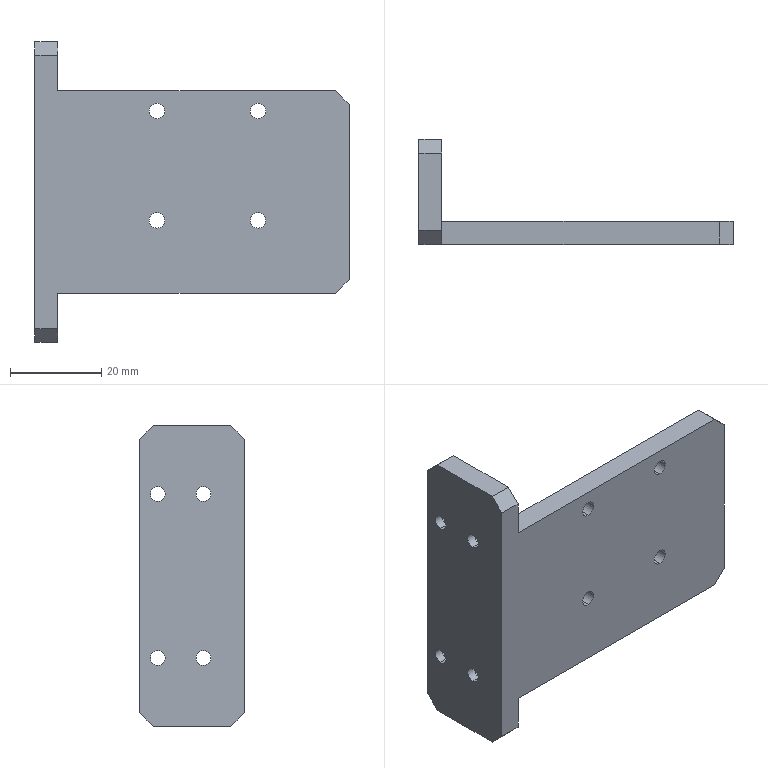Part | STEP file | Guide wheel mechanism revised.sldasm-Part-497 | 1 solid | 44 faces | box 69 x 23 x 66 mm | volume 21162 mm3 | cylinder 24 | plane 20 | commonest cylinder face diameters 3.24 x8 3.4 x8 5.5 x8
STEP:
#1=CARTESIAN_POINT('',(-3.,4.,20.75));
#2=VERTEX_POINT('',#1);
#3=CARTESIAN_POINT('',(-3.,4.,15.25));
#4=VERTEX_POINT('',#3);
#5=CARTESIAN_POINT('',(-3.,4.,18.));
#6=DIRECTION('',(1.,0.,0.));
#7=DIRECTION('',(0.,0.,-1.));
#8=AXIS2_PLACEMENT_3D('',#5,#6,#7);
#9=CIRCLE('',#8,2.75);
#10=EDGE_CURVE('',#2,#4,#9,.T.);
#11=ORIENTED_EDGE('',*,*,#10,.F.);
#12=CARTESIAN_POINT('',(0.,4.,20.75));
#13=VERTEX_POINT('',#12);
#14=CARTESIAN_POINT('',(-3.,4.,20.75));
#15=DIRECTION('',(1.,0.,0.));
#16=VECTOR('',#15,1000.);
#17=LINE('',#14,#16);
#18=EDGE_CURVE('',#2,#13,#17,.T.);
#19=ORIENTED_EDGE('',*,*,#18,.T.);
#20=CARTESIAN_POINT('',(0.,4.,15.25));
#21=VERTEX_POINT('',#20);
#22=CARTESIAN_POINT('',(0.,4.,18.));
#23=DIRECTION('',(1.,0.,0.));
#24=DIRECTION('',(0.,0.,-1.));
#25=AXIS2_PLACEMENT_3D('',#22,#23,#24);
#26=CIRCLE('',#25,2.75);
#27=EDGE_CURVE('',#13,#21,#26,.T.);
#28=ORIENTED_EDGE('',*,*,#27,.T.);
#29=CARTESIAN_POINT('',(-3.,4.,15.25));
#30=DIRECTION('',(1.,0.,0.));
#31=VECTOR('',#30,1000.);
#32=LINE('',#29,#31);
#33=EDGE_CURVE('',#4,#21,#32,.T.);
#34=ORIENTED_EDGE('',*,*,#33,.F.);
#35=EDGE_LOOP('',(#11,#19,#28,#34));
#36=FACE_OUTER_BOUND('',#35,.T.);
#37=CARTESIAN_POINT('',(-3.,4.,18.));
#38=DIRECTION('',(1.,0.,0.));
#39=DIRECTION('',(0.,0.,-1.));
#40=AXIS2_PLACEMENT_3D('',#37,#38,#39);
#41=CYLINDRICAL_SURFACE('',#40,2.75);
#42=ADVANCED_FACE('',(#36),#41,.F.);
#43=CARTESIAN_POINT('',(-3.,4.,-15.25));
#44=VERTEX_POINT('',#43);
#45=CARTESIAN_POINT('',(-3.,4.,-20.75));
#46=VERTEX_POINT('',#45);
#47=CARTESIAN_POINT('',(-3.,4.,-18.));
#48=DIRECTION('',(1.,0.,0.));
#49=DIRECTION('',(0.,0.,-1.));
#50=AXIS2_PLACEMENT_3D('',#47,#48,#49);
#51=CIRCLE('',#50,2.75);
#52=EDGE_CURVE('',#44,#46,#51,.T.);
#53=ORIENTED_EDGE('',*,*,#52,.F.);
#54=CARTESIAN_POINT('',(0.,4.,-15.25));
#55=VERTEX_POINT('',#54);
#56=CARTESIAN_POINT('',(-3.,4.,-15.25));
#57=DIRECTION('',(1.,0.,0.));
#58=VECTOR('',#57,1000.);
#59=LINE('',#56,#58);
#60=EDGE_CURVE('',#44,#55,#59,.T.);
#61=ORIENTED_EDGE('',*,*,#60,.T.);
#62=CARTESIAN_POINT('',(0.,4.,-20.75));
#63=VERTEX_POINT('',#62);
#64=CARTESIAN_POINT('',(0.,4.,-18.));
#65=DIRECTION('',(1.,0.,0.));
#66=DIRECTION('',(0.,0.,-1.));
#67=AXIS2_PLACEMENT_3D('',#64,#65,#66);
#68=CIRCLE('',#67,2.75);
#69=EDGE_CURVE('',#55,#63,#68,.T.);
#70=ORIENTED_EDGE('',*,*,#69,.T.);
#71=CARTESIAN_POINT('',(-3.,4.,-20.75));
#72=DIRECTION('',(1.,0.,0.));
#73=VECTOR('',#72,1000.);
#74=LINE('',#71,#73);
#75=EDGE_CURVE('',#46,#63,#74,.T.);
#76=ORIENTED_EDGE('',*,*,#75,.F.);
#77=EDGE_LOOP('',(#53,#61,#70,#76));
#78=FACE_OUTER_BOUND('',#77,.T.);
#79=CARTESIAN_POINT('',(-3.,4.,-18.));
#80=DIRECTION('',(1.,0.,0.));
#81=DIRECTION('',(0.,0.,-1.));
#82=AXIS2_PLACEMENT_3D('',#79,#80,#81);
#83=CYLINDRICAL_SURFACE('',#82,2.75);
#84=ADVANCED_FACE('',(#78),#83,.F.);
#85=CARTESIAN_POINT('',(-3.,14.,-15.25));
#86=VERTEX_POINT('',#85);
#87=CARTESIAN_POINT('',(-3.,14.,-20.75));
#88=VERTEX_POINT('',#87);
#89=CARTESIAN_POINT('',(-3.,14.,-18.));
#90=DIRECTION('',(1.,0.,0.));
#91=DIRECTION('',(0.,0.,-1.));
#92=AXIS2_PLACEMENT_3D('',#89,#90,#91);
#93=CIRCLE('',#92,2.75);
#94=EDGE_CURVE('',#86,#88,#93,.T.);
#95=ORIENTED_EDGE('',*,*,#94,.F.);
#96=CARTESIAN_POINT('',(0.,14.,-15.25));
#97=VERTEX_POINT('',#96);
#98=CARTESIAN_POINT('',(-3.,14.,-15.25));
#99=DIRECTION('',(1.,0.,0.));
#100=VECTOR('',#99,1000.);
#101=LINE('',#98,#100);
#102=EDGE_CURVE('',#86,#97,#101,.T.);
#103=ORIENTED_EDGE('',*,*,#102,.T.);
#104=CARTESIAN_POINT('',(0.,14.,-20.75));
#105=VERTEX_POINT('',#104);
#106=CARTESIAN_POINT('',(0.,14.,-18.));
#107=DIRECTION('',(1.,0.,0.));
#108=DIRECTION('',(0.,0.,-1.));
#109=AXIS2_PLACEMENT_3D('',#106,#107,#108);
#110=CIRCLE('',#109,2.75);
#111=EDGE_CURVE('',#97,#105,#110,.T.);
#112=ORIENTED_EDGE('',*,*,#111,.T.);
#113=CARTESIAN_POINT('',(-3.,14.,-20.75));
#114=DIRECTION('',(1.,0.,0.));
#115=VECTOR('',#114,1000.);
#116=LINE('',#113,#115);
#117=EDGE_CURVE('',#88,#105,#116,.T.);
#118=ORIENTED_EDGE('',*,*,#117,.F.);
#119=EDGE_LOOP('',(#95,#103,#112,#118));
#120=FACE_OUTER_BOUND('',#119,.T.);
#121=CARTESIAN_POINT('',(-3.,14.,-18.));
#122=DIRECTION('',(1.,0.,0.));
#123=DIRECTION('',(0.,0.,-1.));
#124=AXIS2_PLACEMENT_3D('',#121,#122,#123);
#125=CYLINDRICAL_SURFACE('',#124,2.75);
#126=ADVANCED_FACE('',(#120),#125,.F.);
#127=CARTESIAN_POINT('',(-3.,14.,20.75));
#128=VERTEX_POINT('',#127);
#129=CARTESIAN_POINT('',(-3.,14.,15.25));
#130=VERTEX_POINT('',#129);
#131=CARTESIAN_POINT('',(-3.,14.,18.));
#132=DIRECTION('',(1.,0.,0.));
#133=DIRECTION('',(0.,0.,-1.));
#134=AXIS2_PLACEMENT_3D('',#131,#132,#133);
#135=CIRCLE('',#134,2.75);
#136=EDGE_CURVE('',#128,#130,#135,.T.);
#137=ORIENTED_EDGE('',*,*,#136,.F.);
#138=CARTESIAN_POINT('',(0.,14.,20.75));
#139=VERTEX_POINT('',#138);
#140=CARTESIAN_POINT('',(-3.,14.,20.75));
#141=DIRECTION('',(1.,0.,0.));
#142=VECTOR('',#141,1000.);
#143=LINE('',#140,#142);
#144=EDGE_CURVE('',#128,#139,#143,.T.);
#145=ORIENTED_EDGE('',*,*,#144,.T.);
#146=CARTESIAN_POINT('',(0.,14.,15.25));
#147=VERTEX_POINT('',#146);
#148=CARTESIAN_POINT('',(0.,14.,18.));
#149=DIRECTION('',(1.,0.,0.));
#150=DIRECTION('',(0.,0.,-1.));
#151=AXIS2_PLACEMENT_3D('',#148,#149,#150);
#152=CIRCLE('',#151,2.75);
#153=EDGE_CURVE('',#139,#147,#152,.T.);
#154=ORIENTED_EDGE('',*,*,#153,.T.);
#155=CARTESIAN_POINT('',(-3.,14.,15.25));
#156=DIRECTION('',(1.,0.,0.));
#157=VECTOR('',#156,1000.);
#158=LINE('',#155,#157);
#159=EDGE_CURVE('',#130,#147,#158,.T.);
#160=ORIENTED_EDGE('',*,*,#159,.F.);
#161=EDGE_LOOP('',(#137,#145,#154,#160));
#162=FACE_OUTER_BOUND('',#161,.T.);
#163=CARTESIAN_POINT('',(-3.,14.,18.));
#164=DIRECTION('',(1.,0.,0.));
#165=DIRECTION('',(0.,0.,-1.));
#166=AXIS2_PLACEMENT_3D('',#163,#164,#165);
#167=CYLINDRICAL_SURFACE('',#166,2.75);
#168=ADVANCED_FACE('',(#162),#167,.F.);
#169=CARTESIAN_POINT('',(21.8,-5.,16.05));
#170=VERTEX_POINT('',#169);
#171=CARTESIAN_POINT('',(21.8,-5.,19.45));
#172=VERTEX_POINT('',#171);
#173=CARTESIAN_POINT('',(21.8,-5.,17.75));
#174=DIRECTION('',(0.,1.,0.));
#175=DIRECTION('',(0.,0.,-1.));
#176=AXIS2_PLACEMENT_3D('',#173,#174,#175);
#177=CIRCLE('',#176,1.7);
#178=EDGE_CURVE('',#170,#172,#177,.T.);
#179=ORIENTED_EDGE('',*,*,#178,.F.);
#180=CARTESIAN_POINT('',(21.8,0.,16.05));
#181=VERTEX_POINT('',#180);
#182=CARTESIAN_POINT('',(21.8,-5.001,16.05));
#183=DIRECTION('',(0.,1.,0.));
#184=VECTOR('',#183,1000.);
#185=LINE('',#182,#184);
#186=EDGE_CURVE('',#170,#181,#185,.T.);
#187=ORIENTED_EDGE('',*,*,#186,.T.);
#188=CARTESIAN_POINT('',(21.8,0.,19.45));
#189=VERTEX_POINT('',#188);
#190=CARTESIAN_POINT('',(21.8,0.,17.75));
#191=DIRECTION('',(0.,1.,0.));
#192=DIRECTION('',(0.,0.,1.));
#193=AXIS2_PLACEMENT_3D('',#190,#191,#192);
#194=CIRCLE('',#193,1.7);
#195=EDGE_CURVE('',#181,#189,#194,.T.);
#196=ORIENTED_EDGE('',*,*,#195,.T.);
#197=CARTESIAN_POINT('',(21.8,-5.001,19.45));
#198=DIRECTION('',(0.,1.,0.));
#199=VECTOR('',#198,1000.);
#200=LINE('',#197,#199);
#201=EDGE_CURVE('',#172,#189,#200,.T.);
#202=ORIENTED_EDGE('',*,*,#201,.F.);
#203=EDGE_LOOP('',(#179,#187,#196,#202));
#204=FACE_OUTER_BOUND('',#203,.T.);
#205=CARTESIAN_POINT('',(21.8,-5.001,17.75));
#206=DIRECTION('',(0.,1.,0.));
#207=DIRECTION('',(0.,0.,1.));
#208=AXIS2_PLACEMENT_3D('',#205,#206,#207);
#209=CYLINDRICAL_SURFACE('',#208,1.7);
#210=ADVANCED_FACE('',(#204),#209,.F.);
#211=CARTESIAN_POINT('',(44.,-5.,16.05));
#212=VERTEX_POINT('',#211);
#213=CARTESIAN_POINT('',(44.,-5.,19.45));
#214=VERTEX_POINT('',#213);
#215=CARTESIAN_POINT('',(44.,-5.,17.75));
#216=DIRECTION('',(0.,1.,0.));
#217=DIRECTION('',(0.,0.,-1.));
#218=AXIS2_PLACEMENT_3D('',#215,#216,#217);
#219=CIRCLE('',#218,1.7);
#220=EDGE_CURVE('',#212,#214,#219,.T.);
#221=ORIENTED_EDGE('',*,*,#220,.F.);
#222=CARTESIAN_POINT('',(44.,0.,16.05));
#223=VERTEX_POINT('',#222);
#224=CARTESIAN_POINT('',(44.,-5.001,16.05));
#225=DIRECTION('',(0.,1.,0.));
#226=VECTOR('',#225,1000.);
#227=LINE('',#224,#226);
#228=EDGE_CURVE('',#212,#223,#227,.T.);
#229=ORIENTED_EDGE('',*,*,#228,.T.);
#230=CARTESIAN_POINT('',(44.,0.,19.45));
#231=VERTEX_POINT('',#230);
#232=CARTESIAN_POINT('',(44.,0.,17.75));
#233=DIRECTION('',(0.,1.,0.));
#234=DIRECTION('',(0.,0.,1.));
#235=AXIS2_PLACEMENT_3D('',#232,#233,#234);
#236=CIRCLE('',#235,1.7);
#237=EDGE_CURVE('',#223,#231,#236,.T.);
#238=ORIENTED_EDGE('',*,*,#237,.T.);
#239=CARTESIAN_POINT('',(44.,-5.001,19.45));
#240=DIRECTION('',(0.,1.,0.));
#241=VECTOR('',#240,1000.);
#242=LINE('',#239,#241);
#243=EDGE_CURVE('',#214,#231,#242,.T.);
#244=ORIENTED_EDGE('',*,*,#243,.F.);
#245=EDGE_LOOP('',(#221,#229,#238,#244));
#246=FACE_OUTER_BOUND('',#245,.T.);
#247=CARTESIAN_POINT('',(44.,-5.001,17.75));
#248=DIRECTION('',(0.,1.,0.));
#249=DIRECTION('',(0.,0.,1.));
#250=AXIS2_PLACEMENT_3D('',#247,#248,#249);
#251=CYLINDRICAL_SURFACE('',#250,1.7);
#252=ADVANCED_FACE('',(#246),#251,.F.);
#253=CARTESIAN_POINT('',(44.,-5.,-7.95));
#254=VERTEX_POINT('',#253);
#255=CARTESIAN_POINT('',(44.,-5.,-4.55));
#256=VERTEX_POINT('',#255);
#257=CARTESIAN_POINT('',(44.,-5.,-6.25));
#258=DIRECTION('',(0.,1.,0.));
#259=DIRECTION('',(0.,0.,-1.));
#260=AXIS2_PLACEMENT_3D('',#257,#258,#259);
#261=CIRCLE('',#260,1.7);
#262=EDGE_CURVE('',#254,#256,#261,.T.);
#263=ORIENTED_EDGE('',*,*,#262,.F.);
#264=CARTESIAN_POINT('',(44.,0.,-7.95));
#265=VERTEX_POINT('',#264);
#266=CARTESIAN_POINT('',(44.,-5.001,-7.95));
#267=DIRECTION('',(0.,1.,0.));
#268=VECTOR('',#267,1000.);
#269=LINE('',#266,#268);
#270=EDGE_CURVE('',#254,#265,#269,.T.);
#271=ORIENTED_EDGE('',*,*,#270,.T.);
#272=CARTESIAN_POINT('',(44.,0.,-4.55));
#273=VERTEX_POINT('',#272);
#274=CARTESIAN_POINT('',(44.,0.,-6.25));
#275=DIRECTION('',(0.,1.,0.));
#276=DIRECTION('',(0.,0.,1.));
#277=AXIS2_PLACEMENT_3D('',#274,#275,#276);
#278=CIRCLE('',#277,1.7);
#279=EDGE_CURVE('',#265,#273,#278,.T.);
#280=ORIENTED_EDGE('',*,*,#279,.T.);
#281=CARTESIAN_POINT('',(44.,-5.001,-4.55));
#282=DIRECTION('',(0.,1.,0.));
#283=VECTOR('',#282,1000.);
#284=LINE('',#281,#283);
#285=EDGE_CURVE('',#256,#273,#284,.T.);
#286=ORIENTED_EDGE('',*,*,#285,.F.);
#287=EDGE_LOOP('',(#263,#271,#280,#286));
#288=FACE_OUTER_BOUND('',#287,.T.);
#289=CARTESIAN_POINT('',(44.,-5.001,-6.25));
#290=DIRECTION('',(0.,1.,0.));
#291=DIRECTION('',(0.,0.,1.));
#292=AXIS2_PLACEMENT_3D('',#289,#290,#291);
#293=CYLINDRICAL_SURFACE('',#292,1.7);
#294=ADVANCED_FACE('',(#288),#293,.F.);
#295=CARTESIAN_POINT('',(21.8,-5.,-7.95));
#296=VERTEX_POINT('',#295);
#297=CARTESIAN_POINT('',(21.8,-5.,-4.55));
#298=VERTEX_POINT('',#297);
#299=CARTESIAN_POINT('',(21.8,-5.,-6.25));
#300=DIRECTION('',(0.,1.,0.));
#301=DIRECTION('',(0.,0.,-1.));
#302=AXIS2_PLACEMENT_3D('',#299,#300,#301);
#303=CIRCLE('',#302,1.7);
#304=EDGE_CURVE('',#296,#298,#303,.T.);
#305=ORIENTED_EDGE('',*,*,#304,.F.);
#306=CARTESIAN_POINT('',(21.8,0.,-7.95));
#307=VERTEX_POINT('',#306);
#308=CARTESIAN_POINT('',(21.8,-5.001,-7.95));
#309=DIRECTION('',(0.,1.,0.));
#310=VECTOR('',#309,1000.);
#311=LINE('',#308,#310);
#312=EDGE_CURVE('',#296,#307,#311,.T.);
#313=ORIENTED_EDGE('',*,*,#312,.T.);
#314=CARTESIAN_POINT('',(21.8,0.,-4.55));
#315=VERTEX_POINT('',#314);
#316=CARTESIAN_POINT('',(21.8,0.,-6.25));
#317=DIRECTION('',(0.,1.,0.));
#318=DIRECTION('',(0.,0.,1.));
#319=AXIS2_PLACEMENT_3D('',#316,#317,#318);
#320=CIRCLE('',#319,1.7);
#321=EDGE_CURVE('',#307,#315,#320,.T.);
#322=ORIENTED_EDGE('',*,*,#321,.T.);
#323=CARTESIAN_POINT('',(21.8,-5.001,-4.55));
#324=DIRECTION('',(0.,1.,0.));
#325=VECTOR('',#324,1000.);
#326=LINE('',#323,#325);
#327=EDGE_CURVE('',#298,#315,#326,.T.);
#328=ORIENTED_EDGE('',*,*,#327,.F.);
#329=EDGE_LOOP('',(#305,#313,#322,#328));
#330=FACE_OUTER_BOUND('',#329,.T.);
#331=CARTESIAN_POINT('',(21.8,-5.001,-6.25));
#332=DIRECTION('',(0.,1.,0.));
#333=DIRECTION('',(0.,0.,1.));
#334=AXIS2_PLACEMENT_3D('',#331,#332,#333);
#335=CYLINDRICAL_SURFACE('',#334,1.7);
#336=ADVANCED_FACE('',(#330),#335,.F.);
#337=CARTESIAN_POINT('',(-5.,14.,19.62));
#338=VERTEX_POINT('',#337);
#339=CARTESIAN_POINT('',(-5.,14.,16.38));
#340=VERTEX_POINT('',#339);
#341=CARTESIAN_POINT('',(-5.,14.,18.));
#342=DIRECTION('',(1.,0.,0.));
#343=DIRECTION('',(0.,0.,1.));
#344=AXIS2_PLACEMENT_3D('',#341,#342,#343);
#345=CIRCLE('',#344,1.62);
#346=EDGE_CURVE('',#338,#340,#345,.T.);
#347=ORIENTED_EDGE('',*,*,#346,.F.);
#348=CARTESIAN_POINT('',(-3.,14.,19.62));
#349=VERTEX_POINT('',#348);
#350=CARTESIAN_POINT('',(-5.001,14.,19.62));
#351=DIRECTION('',(1.,0.,0.));
#352=VECTOR('',#351,1000.);
#353=LINE('',#350,#352);
#354=EDGE_CURVE('',#338,#349,#353,.T.);
#355=ORIENTED_EDGE('',*,*,#354,.T.);
#356=CARTESIAN_POINT('',(-3.,14.,16.38));
#357=VERTEX_POINT('',#356);
#358=CARTESIAN_POINT('',(-3.,14.,18.));
#359=DIRECTION('',(-1.,0.,0.));
#360=DIRECTION('',(0.,0.,-1.));
#361=AXIS2_PLACEMENT_3D('',#358,#359,#360);
#362=CIRCLE('',#361,1.62);
#363=EDGE_CURVE('',#357,#349,#362,.T.);
#364=ORIENTED_EDGE('',*,*,#363,.F.);
#365=CARTESIAN_POINT('',(-5.001,14.,16.38));
#366=DIRECTION('',(1.,0.,0.));
#367=VECTOR('',#366,1000.);
#368=LINE('',#365,#367);
#369=EDGE_CURVE('',#340,#357,#368,.T.);
#370=ORIENTED_EDGE('',*,*,#369,.F.);
#371=EDGE_LOOP('',(#347,#355,#364,#370));
#372=FACE_OUTER_BOUND('',#371,.T.);
#373=CARTESIAN_POINT('',(-5.001,14.,18.));
#374=DIRECTION('',(1.,0.,0.));
#375=DIRECTION('',(0.,0.,-1.));
#376=AXIS2_PLACEMENT_3D('',#373,#374,#375);
#377=CYLINDRICAL_SURFACE('',#376,1.62);
#378=ADVANCED_FACE('',(#372),#377,.F.);
#379=CARTESIAN_POINT('',(-5.,14.,-16.38));
#380=VERTEX_POINT('',#379);
#381=CARTESIAN_POINT('',(-5.,14.,-19.62));
#382=VERTEX_POINT('',#381);
#383=CARTESIAN_POINT('',(-5.,14.,-18.));
#384=DIRECTION('',(1.,0.,0.));
#385=DIRECTION('',(0.,0.,1.));
#386=AXIS2_PLACEMENT_3D('',#383,#384,#385);
#387=CIRCLE('',#386,1.62);
#388=EDGE_CURVE('',#380,#382,#387,.T.);
#389=ORIENTED_EDGE('',*,*,#388,.F.);
#390=CARTESIAN_POINT('',(-3.,14.,-16.38));
#391=VERTEX_POINT('',#390);
#392=CARTESIAN_POINT('',(-5.001,14.,-16.38));
#393=DIRECTION('',(1.,0.,0.));
#394=VECTOR('',#393,1000.);
#395=LINE('',#392,#394);
#396=EDGE_CURVE('',#380,#391,#395,.T.);
#397=ORIENTED_EDGE('',*,*,#396,.T.);
#398=CARTESIAN_POINT('',(-3.,14.,-19.62));
#399=VERTEX_POINT('',#398);
#400=CARTESIAN_POINT('',(-3.,14.,-18.));
#401=DIRECTION('',(-1.,0.,0.));
#402=DIRECTION('',(0.,0.,-1.));
#403=AXIS2_PLACEMENT_3D('',#400,#401,#402);
#404=CIRCLE('',#403,1.62);
#405=EDGE_CURVE('',#399,#391,#404,.T.);
#406=ORIENTED_EDGE('',*,*,#405,.F.);
#407=CARTESIAN_POINT('',(-5.001,14.,-19.62));
#408=DIRECTION('',(1.,0.,0.));
#409=VECTOR('',#408,1000.);
#410=LINE('',#407,#409);
#411=EDGE_CURVE('',#382,#399,#410,.T.);
#412=ORIENTED_EDGE('',*,*,#411,.F.);
#413=EDGE_LOOP('',(#389,#397,#406,#412));
#414=FACE_OUTER_BOUND('',#413,.T.);
#415=CARTESIAN_POINT('',(-5.001,14.,-18.));
#416=DIRECTION('',(1.,0.,0.));
#417=DIRECTION('',(0.,0.,-1.));
#418=AXIS2_PLACEMENT_3D('',#415,#416,#417);
#419=CYLINDRICAL_SURFACE('',#418,1.62);
#420=ADVANCED_FACE('',(#414),#419,.F.);
#421=CARTESIAN_POINT('',(-5.,4.,-16.38));
#422=VERTEX_POINT('',#421);
#423=CARTESIAN_POINT('',(-5.,4.,-19.62));
#424=VERTEX_POINT('',#423);
#425=CARTESIAN_POINT('',(-5.,4.,-18.));
#426=DIRECTION('',(1.,0.,0.));
#427=DIRECTION('',(0.,0.,1.));
#428=AXIS2_PLACEMENT_3D('',#425,#426,#427);
#429=CIRCLE('',#428,1.62);
#430=EDGE_CURVE('',#422,#424,#429,.T.);
#431=ORIENTED_EDGE('',*,*,#430,.F.);
#432=CARTESIAN_POINT('',(-3.,4.,-16.38));
#433=VERTEX_POINT('',#432);
#434=CARTESIAN_POINT('',(-5.001,4.,-16.38));
#435=DIRECTION('',(1.,0.,0.));
#436=VECTOR('',#435,1000.);
#437=LINE('',#434,#436);
#438=EDGE_CURVE('',#422,#433,#437,.T.);
#439=ORIENTED_EDGE('',*,*,#438,.T.);
#440=CARTESIAN_POINT('',(-3.,4.,-19.62));
#441=VERTEX_POINT('',#440);
#442=CARTESIAN_POINT('',(-3.,4.,-18.));
#443=DIRECTION('',(-1.,0.,0.));
#444=DIRECTION('',(0.,0.,-1.));
#445=AXIS2_PLACEMENT_3D('',#442,#443,#444);
#446=CIRCLE('',#445,1.62);
#447=EDGE_CURVE('',#441,#433,#446,.T.);
#448=ORIENTED_EDGE('',*,*,#447,.F.);
#449=CARTESIAN_POINT('',(-5.001,4.,-19.62));
#450=DIRECTION('',(1.,0.,0.));
#451=VECTOR('',#450,1000.);
#452=LINE('',#449,#451);
#453=EDGE_CURVE('',#424,#441,#452,.T.);
#454=ORIENTED_EDGE('',*,*,#453,.F.);
#455=EDGE_LOOP('',(#431,#439,#448,#454));
#456=FACE_OUTER_BOUND('',#455,.T.);
#457=CARTESIAN_POINT('',(-5.001,4.,-18.));
#458=DIRECTION('',(1.,0.,0.));
#459=DIRECTION('',(0.,0.,-1.));
#460=AXIS2_PLACEMENT_3D('',#457,#458,#459);
#461=CYLINDRICAL_SURFACE('',#460,1.62);
#462=ADVANCED_FACE('',(#456),#461,.F.);
#463=CARTESIAN_POINT('',(-5.,4.,19.62));
#464=VERTEX_POINT('',#463);
#465=CARTESIAN_POINT('',(-5.,4.,16.38));
#466=VERTEX_POINT('',#465);
#467=CARTESIAN_POINT('',(-5.,4.,18.));
#468=DIRECTION('',(1.,0.,0.));
#469=DIRECTION('',(0.,0.,1.));
#470=AXIS2_PLACEMENT_3D('',#467,#468,#469);
#471=CIRCLE('',#470,1.62);
#472=EDGE_CURVE('',#464,#466,#471,.T.);
#473=ORIENTED_EDGE('',*,*,#472,.F.);
#474=CARTESIAN_POINT('',(-3.,4.,19.62));
#475=VERTEX_POINT('',#474);
#476=CARTESIAN_POINT('',(-5.001,4.,19.62));
#477=DIRECTION('',(1.,0.,0.));
#478=VECTOR('',#477,1000.);
#479=LINE('',#476,#478);
#480=EDGE_CURVE('',#464,#475,#479,.T.);
#481=ORIENTED_EDGE('',*,*,#480,.T.);
#482=CARTESIAN_POINT('',(-3.,4.,16.38));
#483=VERTEX_POINT('',#482);
#484=CARTESIAN_POINT('',(-3.,4.,18.));
#485=DIRECTION('',(-1.,0.,0.));
#486=DIRECTION('',(0.,0.,-1.));
#487=AXIS2_PLACEMENT_3D('',#484,#485,#486);
#488=CIRCLE('',#487,1.62);
#489=EDGE_CURVE('',#483,#475,#488,.T.);
#490=ORIENTED_EDGE('',*,*,#489,.F.);
#491=CARTESIAN_POINT('',(-5.001,4.,16.38));
#492=DIRECTION('',(1.,0.,0.));
#493=VECTOR('',#492,1000.);
#494=LINE('',#491,#493);
#495=EDGE_CURVE('',#466,#483,#494,.T.);
#496=ORIENTED_EDGE('',*,*,#495,.F.);
#497=EDGE_LOOP('',(#473,#481,#490,#496));
#498=FACE_OUTER_BOUND('',#497,.T.);
#499=CARTESIAN_POINT('',(-5.001,4.,18.));
#500=DIRECTION('',(1.,0.,0.));
#501=DIRECTION('',(0.,0.,-1.));
#502=AXIS2_PLACEMENT_3D('',#499,#500,#501);
#503=CYLINDRICAL_SURFACE('',#502,1.62);
#504=ADVANCED_FACE('',(#498),#503,.F.);
#505=ORIENTED_EDGE('',*,*,#480,.F.);
#506=CARTESIAN_POINT('',(-5.,4.,18.));
#507=DIRECTION('',(1.,0.,0.));
#508=DIRECTION('',(0.,0.,1.));
#509=AXIS2_PLACEMENT_3D('',#506,#507,#508);
#510=CIRCLE('',#509,1.62);
#511=EDGE_CURVE('',#466,#464,#510,.T.);
#512=ORIENTED_EDGE('',*,*,#511,.F.);
#513=ORIENTED_EDGE('',*,*,#495,.T.);
#514=CARTESIAN_POINT('',(-3.,4.,18.));
#515=DIRECTION('',(-1.,0.,0.));
#516=DIRECTION('',(0.,0.,-1.));
#517=AXIS2_PLACEMENT_3D('',#514,#515,#516);
#518=CIRCLE('',#517,1.62);
#519=EDGE_CURVE('',#475,#483,#518,.T.);
#520=ORIENTED_EDGE('',*,*,#519,.F.);
#521=EDGE_LOOP('',(#505,#512,#513,#520));
#522=FACE_OUTER_BOUND('',#521,.T.);
#523=CARTESIAN_POINT('',(-5.001,4.,18.));
#524=DIRECTION('',(1.,0.,0.));
#525=DIRECTION('',(0.,0.,-1.));
#526=AXIS2_PLACEMENT_3D('',#523,#524,#525);
#527=CYLINDRICAL_SURFACE('',#526,1.62);
#528=ADVANCED_FACE('',(#522),#527,.F.);
#529=ORIENTED_EDGE('',*,*,#438,.F.);
#530=CARTESIAN_POINT('',(-5.,4.,-18.));
#531=DIRECTION('',(1.,0.,0.));
#532=DIRECTION('',(0.,0.,1.));
#533=AXIS2_PLACEMENT_3D('',#530,#531,#532);
#534=CIRCLE('',#533,1.62);
#535=EDGE_CURVE('',#424,#422,#534,.T.);
#536=ORIENTED_EDGE('',*,*,#535,.F.);
#537=ORIENTED_EDGE('',*,*,#453,.T.);
#538=CARTESIAN_POINT('',(-3.,4.,-18.));
#539=DIRECTION('',(-1.,0.,0.));
#540=DIRECTION('',(0.,0.,-1.));
#541=AXIS2_PLACEMENT_3D('',#538,#539,#540);
#542=CIRCLE('',#541,1.62);
#543=EDGE_CURVE('',#433,#441,#542,.T.);
#544=ORIENTED_EDGE('',*,*,#543,.F.);
#545=EDGE_LOOP('',(#529,#536,#537,#544));
#546=FACE_OUTER_BOUND('',#545,.T.);
#547=CARTESIAN_POINT('',(-5.001,4.,-18.));
#548=DIRECTION('',(1.,0.,0.));
#549=DIRECTION('',(0.,0.,-1.));
#550=AXIS2_PLACEMENT_3D('',#547,#548,#549);
#551=CYLINDRICAL_SURFACE('',#550,1.62);
#552=ADVANCED_FACE('',(#546),#551,.F.);
#553=ORIENTED_EDGE('',*,*,#396,.F.);
#554=CARTESIAN_POINT('',(-5.,14.,-18.));
#555=DIRECTION('',(1.,0.,0.));
#556=DIRECTION('',(0.,0.,1.));
#557=AXIS2_PLACEMENT_3D('',#554,#555,#556);
#558=CIRCLE('',#557,1.62);
#559=EDGE_CURVE('',#382,#380,#558,.T.);
#560=ORIENTED_EDGE('',*,*,#559,.F.);
#561=ORIENTED_EDGE('',*,*,#411,.T.);
#562=CARTESIAN_POINT('',(-3.,14.,-18.));
#563=DIRECTION('',(-1.,0.,0.));
#564=DIRECTION('',(0.,0.,-1.));
#565=AXIS2_PLACEMENT_3D('',#562,#563,#564);
#566=CIRCLE('',#565,1.62);
#567=EDGE_CURVE('',#391,#399,#566,.T.);
#568=ORIENTED_EDGE('',*,*,#567,.F.);
#569=EDGE_LOOP('',(#553,#560,#561,#568));
#570=FACE_OUTER_BOUND('',#569,.T.);
#571=CARTESIAN_POINT('',(-5.001,14.,-18.));
#572=DIRECTION('',(1.,0.,0.));
#573=DIRECTION('',(0.,0.,-1.));
#574=AXIS2_PLACEMENT_3D('',#571,#572,#573);
#575=CYLINDRICAL_SURFACE('',#574,1.62);
#576=ADVANCED_FACE('',(#570),#575,.F.);
#577=ORIENTED_EDGE('',*,*,#354,.F.);
#578=CARTESIAN_POINT('',(-5.,14.,18.));
#579=DIRECTION('',(1.,0.,0.));
#580=DIRECTION('',(0.,0.,1.));
#581=AXIS2_PLACEMENT_3D('',#578,#579,#580);
#582=CIRCLE('',#581,1.62);
#583=EDGE_CURVE('',#340,#338,#582,.T.);
#584=ORIENTED_EDGE('',*,*,#583,.F.);
#585=ORIENTED_EDGE('',*,*,#369,.T.);
#586=CARTESIAN_POINT('',(-3.,14.,18.));
#587=DIRECTION('',(-1.,0.,0.));
#588=DIRECTION('',(0.,0.,-1.));
#589=AXIS2_PLACEMENT_3D('',#586,#587,#588);
#590=CIRCLE('',#589,1.62);
#591=EDGE_CURVE('',#349,#357,#590,.T.);
#592=ORIENTED_EDGE('',*,*,#591,.F.);
#593=EDGE_LOOP('',(#577,#584,#585,#592));
#594=FACE_OUTER_BOUND('',#593,.T.);
#595=CARTESIAN_POINT('',(-5.001,14.,18.));
#596=DIRECTION('',(1.,0.,0.));
#597=DIRECTION('',(0.,0.,-1.));
#598=AXIS2_PLACEMENT_3D('',#595,#596,#597);
#599=CYLINDRICAL_SURFACE('',#598,1.62);
#600=ADVANCED_FACE('',(#594),#599,.F.);
#601=CARTESIAN_POINT('',(21.8,-5.,17.75));
#602=DIRECTION('',(0.,1.,0.));
#603=DIRECTION('',(0.,0.,-1.));
#604=AXIS2_PLACEMENT_3D('',#601,#602,#603);
#605=CIRCLE('',#604,1.7);
#606=EDGE_CURVE('',#172,#170,#605,.T.);
#607=ORIENTED_EDGE('',*,*,#606,.T.);
#608=ORIENTED_EDGE('',*,*,#178,.T.);
#609=EDGE_LOOP('',(#607,#608));
#610=FACE_BOUND('',#609,.T.);
#611=CARTESIAN_POINT('',(44.,-5.,17.75));
#612=DIRECTION('',(0.,1.,0.));
#613=DIRECTION('',(0.,0.,-1.));
#614=AXIS2_PLACEMENT_3D('',#611,#612,#613);
#615=CIRCLE('',#614,1.7);
#616=EDGE_CURVE('',#214,#212,#615,.T.);
#617=ORIENTED_EDGE('',*,*,#616,.T.);
#618=ORIENTED_EDGE('',*,*,#220,.T.);
#619=EDGE_LOOP('',(#617,#618));
#620=FACE_BOUND('',#619,.T.);
#621=CARTESIAN_POINT('',(44.,-5.,-6.25));
#622=DIRECTION('',(0.,1.,0.));
#623=DIRECTION('',(0.,0.,-1.));
#624=AXIS2_PLACEMENT_3D('',#621,#622,#623);
#625=CIRCLE('',#624,1.7);
#626=EDGE_CURVE('',#256,#254,#625,.T.);
#627=ORIENTED_EDGE('',*,*,#626,.T.);
#628=ORIENTED_EDGE('',*,*,#262,.T.);
#629=EDGE_LOOP('',(#627,#628));
#630=FACE_BOUND('',#629,.T.);
#631=CARTESIAN_POINT('',(21.8,-5.,-6.25));
#632=DIRECTION('',(0.,1.,0.));
#633=DIRECTION('',(0.,0.,-1.));
#634=AXIS2_PLACEMENT_3D('',#631,#632,#633);
#635=CIRCLE('',#634,1.7);
#636=EDGE_CURVE('',#298,#296,#635,.T.);
#637=ORIENTED_EDGE('',*,*,#636,.T.);
#638=ORIENTED_EDGE('',*,*,#304,.T.);
#639=EDGE_LOOP('',(#637,#638));
#640=FACE_BOUND('',#639,.T.);
#641=CARTESIAN_POINT('',(0.,-5.,22.25));
#642=VERTEX_POINT('',#641);
#643=CARTESIAN_POINT('',(0.,-5.,30.));
#644=VERTEX_POINT('',#643);
#645=CARTESIAN_POINT('',(0.,-5.,22.25));
#646=DIRECTION('',(0.,0.,1.));
#647=VECTOR('',#646,1000.);
#648=LINE('',#645,#647);
#649=EDGE_CURVE('',#642,#644,#648,.T.);
#650=ORIENTED_EDGE('',*,*,#649,.T.);
#651=CARTESIAN_POINT('',(-5.,-5.,30.));
#652=VERTEX_POINT('',#651);
#653=CARTESIAN_POINT('',(-5.,-5.,30.));
#654=DIRECTION('',(-1.,0.,0.));
#655=VECTOR('',#654,1000.);
#656=LINE('',#653,#655);
#657=EDGE_CURVE('',#644,#652,#656,.T.);
#658=ORIENTED_EDGE('',*,*,#657,.T.);
#659=CARTESIAN_POINT('',(-5.,-5.,-30.));
#660=VERTEX_POINT('',#659);
#661=CARTESIAN_POINT('',(-5.,-5.,-33.));
#662=DIRECTION('',(0.,0.,1.));
#663=VECTOR('',#662,1000.);
#664=LINE('',#661,#663);
#665=EDGE_CURVE('',#660,#652,#664,.T.);
#666=ORIENTED_EDGE('',*,*,#665,.F.);
#667=CARTESIAN_POINT('',(0.,-5.,-30.));
#668=VERTEX_POINT('',#667);
#669=CARTESIAN_POINT('',(0.,-5.,-30.));
#670=DIRECTION('',(1.,0.,0.));
#671=VECTOR('',#670,1000.);
#672=LINE('',#669,#671);
#673=EDGE_CURVE('',#660,#668,#672,.T.);
#674=ORIENTED_EDGE('',*,*,#673,.T.);
#675=CARTESIAN_POINT('',(0.,-5.,-22.25));
#676=VERTEX_POINT('',#675);
#677=CARTESIAN_POINT('',(0.,-5.,-22.25));
#678=DIRECTION('',(0.,0.,1.));
#679=VECTOR('',#678,1000.);
#680=LINE('',#677,#679);
#681=EDGE_CURVE('',#668,#676,#680,.T.);
#682=ORIENTED_EDGE('',*,*,#681,.T.);
#683=CARTESIAN_POINT('',(61.,-5.,-22.25));
#684=VERTEX_POINT('',#683);
#685=CARTESIAN_POINT('',(64.,-5.,-22.25));
#686=DIRECTION('',(1.,0.,0.));
#687=VECTOR('',#686,1000.);
#688=LINE('',#685,#687);
#689=EDGE_CURVE('',#676,#684,#688,.T.);
#690=ORIENTED_EDGE('',*,*,#689,.T.);
#691=CARTESIAN_POINT('',(64.,-5.,-19.25));
#692=VERTEX_POINT('',#691);
#693=CARTESIAN_POINT('',(25.125,-5.,-58.125));
#694=DIRECTION('',(0.7071,0.,0.7071));
#695=VECTOR('',#694,1000.);
#696=LINE('',#693,#695);
#697=EDGE_CURVE('',#684,#692,#696,.T.);
#698=ORIENTED_EDGE('',*,*,#697,.T.);
#699=CARTESIAN_POINT('',(64.,-5.,19.25));
#700=VERTEX_POINT('',#699);
#701=CARTESIAN_POINT('',(64.,-5.,-33.));
#702=DIRECTION('',(0.,0.,1.));
#703=VECTOR('',#702,1000.);
#704=LINE('',#701,#703);
#705=EDGE_CURVE('',#692,#700,#704,.T.);
#706=ORIENTED_EDGE('',*,*,#705,.T.);
#707=CARTESIAN_POINT('',(61.,-5.,22.25));
#708=VERTEX_POINT('',#707);
#709=CARTESIAN_POINT('',(58.125,-5.,25.125));
#710=DIRECTION('',(-0.7071,0.,0.7071));
#711=VECTOR('',#710,1000.);
#712=LINE('',#709,#711);
#713=EDGE_CURVE('',#700,#708,#712,.T.);
#714=ORIENTED_EDGE('',*,*,#713,.T.);
#715=CARTESIAN_POINT('',(64.,-5.,22.25));
#716=DIRECTION('',(-1.,0.,0.));
#717=VECTOR('',#716,1000.);
#718=LINE('',#715,#717);
#719=EDGE_CURVE('',#708,#642,#718,.T.);
#720=ORIENTED_EDGE('',*,*,#719,.T.);
#721=EDGE_LOOP('',(#650,#658,#666,#674,#682,#690,#698,#706,#714,#720));
#722=FACE_OUTER_BOUND('',#721,.T.);
#723=CARTESIAN_POINT('',(0.,-5.,-33.));
#724=DIRECTION('',(0.,-1.,0.));
#725=DIRECTION('',(0.,0.,-1.));
#726=AXIS2_PLACEMENT_3D('',#723,#724,#725);
#727=PLANE('',#726);
#728=ADVANCED_FACE('',(#610,#620,#630,#640,#722),#727,.T.);
#729=ORIENTED_EDGE('',*,*,#511,.T.);
#730=ORIENTED_EDGE('',*,*,#472,.T.);
#731=EDGE_LOOP('',(#729,#730));
#732=FACE_BOUND('',#731,.T.);
#733=ORIENTED_EDGE('',*,*,#535,.T.);
#734=ORIENTED_EDGE('',*,*,#430,.T.);
#735=EDGE_LOOP('',(#733,#734));
#736=FACE_BOUND('',#735,.T.);
#737=ORIENTED_EDGE('',*,*,#559,.T.);
#738=ORIENTED_EDGE('',*,*,#388,.T.);
#739=EDGE_LOOP('',(#737,#738));
#740=FACE_BOUND('',#739,.T.);
#741=ORIENTED_EDGE('',*,*,#583,.T.);
#742=ORIENTED_EDGE('',*,*,#346,.T.);
#743=EDGE_LOOP('',(#741,#742));
#744=FACE_BOUND('',#743,.T.);
#745=ORIENTED_EDGE('',*,*,#665,.T.);
#746=CARTESIAN_POINT('',(-5.,-2.,33.));
#747=VERTEX_POINT('',#746);
#748=CARTESIAN_POINT('',(-5.,-34.,1.));
#749=DIRECTION('',(0.,0.7071,0.7071));
#750=VECTOR('',#749,1000.);
#751=LINE('',#748,#750);
#752=EDGE_CURVE('',#652,#747,#751,.T.);
#753=ORIENTED_EDGE('',*,*,#752,.T.);
#754=CARTESIAN_POINT('',(-5.,15.,33.));
#755=VERTEX_POINT('',#754);
#756=CARTESIAN_POINT('',(-5.,0.,33.));
#757=DIRECTION('',(0.,-1.,0.));
#758=VECTOR('',#757,1000.);
#759=LINE('',#756,#758);
#760=EDGE_CURVE('',#755,#747,#759,.T.);
#761=ORIENTED_EDGE('',*,*,#760,.F.);
#762=CARTESIAN_POINT('',(-5.,18.,30.));
#763=VERTEX_POINT('',#762);
#764=CARTESIAN_POINT('',(-5.,40.5,7.5));
#765=DIRECTION('',(0.,0.7071,-0.7071));
#766=VECTOR('',#765,1000.);
#767=LINE('',#764,#766);
#768=EDGE_CURVE('',#755,#763,#767,.T.);
#769=ORIENTED_EDGE('',*,*,#768,.T.);
#770=CARTESIAN_POINT('',(-5.,18.,-30.));
#771=VERTEX_POINT('',#770);
#772=CARTESIAN_POINT('',(-5.,18.,-33.));
#773=DIRECTION('',(0.,0.,1.));
#774=VECTOR('',#773,1000.);
#775=LINE('',#772,#774);
#776=EDGE_CURVE('',#771,#763,#775,.T.);
#777=ORIENTED_EDGE('',*,*,#776,.F.);
#778=CARTESIAN_POINT('',(-5.,15.,-33.));
#779=VERTEX_POINT('',#778);
#780=CARTESIAN_POINT('',(-5.,7.5,-40.5));
#781=DIRECTION('',(0.,-0.7071,-0.7071));
#782=VECTOR('',#781,1000.);
#783=LINE('',#780,#782);
#784=EDGE_CURVE('',#771,#779,#783,.T.);
#785=ORIENTED_EDGE('',*,*,#784,.T.);
#786=CARTESIAN_POINT('',(-5.,-2.,-33.));
#787=VERTEX_POINT('',#786);
#788=CARTESIAN_POINT('',(-5.,0.,-33.));
#789=DIRECTION('',(0.,-1.,0.));
#790=VECTOR('',#789,1000.);
#791=LINE('',#788,#790);
#792=EDGE_CURVE('',#779,#787,#791,.T.);
#793=ORIENTED_EDGE('',*,*,#792,.T.);
#794=CARTESIAN_POINT('',(-5.,-1.,-34.));
#795=DIRECTION('',(0.,-0.7071,0.7071));
#796=VECTOR('',#795,1000.);
#797=LINE('',#794,#796);
#798=EDGE_CURVE('',#787,#660,#797,.T.);
#799=ORIENTED_EDGE('',*,*,#798,.T.);
#800=EDGE_LOOP('',(#745,#753,#761,#769,#777,#785,#793,#799));
#801=FACE_OUTER_BOUND('',#800,.T.);
#802=CARTESIAN_POINT('',(-5.,0.,-33.));
#803=DIRECTION('',(-1.,0.,0.));
#804=DIRECTION('',(0.,0.,1.));
#805=AXIS2_PLACEMENT_3D('',#802,#803,#804);
#806=PLANE('',#805);
#807=ADVANCED_FACE('',(#732,#736,#740,#744,#801),#806,.T.);
#808=ORIENTED_EDGE('',*,*,#776,.T.);
#809=CARTESIAN_POINT('',(0.,18.,30.));
#810=VERTEX_POINT('',#809);
#811=CARTESIAN_POINT('',(-5.,18.,30.));
#812=DIRECTION('',(1.,0.,0.));
#813=VECTOR('',#812,1000.);
#814=LINE('',#811,#813);
#815=EDGE_CURVE('',#763,#810,#814,.T.);
#816=ORIENTED_EDGE('',*,*,#815,.T.);
#817=CARTESIAN_POINT('',(0.,18.,-30.));
#818=VERTEX_POINT('',#817);
#819=CARTESIAN_POINT('',(0.,18.,-33.));
#820=DIRECTION('',(0.,0.,1.));
#821=VECTOR('',#820,1000.);
#822=LINE('',#819,#821);
#823=EDGE_CURVE('',#818,#810,#822,.T.);
#824=ORIENTED_EDGE('',*,*,#823,.F.);
#825=CARTESIAN_POINT('',(-5.,18.,-30.));
#826=DIRECTION('',(-1.,0.,0.));
#827=VECTOR('',#826,1000.);
#828=LINE('',#825,#827);
#829=EDGE_CURVE('',#818,#771,#828,.T.);
#830=ORIENTED_EDGE('',*,*,#829,.T.);
#831=EDGE_LOOP('',(#808,#816,#824,#830));
#832=FACE_OUTER_BOUND('',#831,.T.);
#833=CARTESIAN_POINT('',(-5.,18.,-33.));
#834=DIRECTION('',(0.,-1.,0.));
#835=DIRECTION('',(0.,0.,-1.));
#836=AXIS2_PLACEMENT_3D('',#833,#834,#835);
#837=PLANE('',#836);
#838=ADVANCED_FACE('',(#832),#837,.F.);
#839=CARTESIAN_POINT('',(0.,4.,18.));
#840=DIRECTION('',(1.,0.,0.));
#841=DIRECTION('',(0.,0.,-1.));
#842=AXIS2_PLACEMENT_3D('',#839,#840,#841);
#843=CIRCLE('',#842,2.75);
#844=EDGE_CURVE('',#21,#13,#843,.T.);
#845=ORIENTED_EDGE('',*,*,#844,.F.);
#846=ORIENTED_EDGE('',*,*,#27,.F.);
#847=EDGE_LOOP('',(#845,#846));
#848=FACE_BOUND('',#847,.T.);
#849=CARTESIAN_POINT('',(0.,4.,-18.));
#850=DIRECTION('',(1.,0.,0.));
#851=DIRECTION('',(0.,0.,-1.));
#852=AXIS2_PLACEMENT_3D('',#849,#850,#851);
#853=CIRCLE('',#852,2.75);
#854=EDGE_CURVE('',#63,#55,#853,.T.);
#855=ORIENTED_EDGE('',*,*,#854,.F.);
#856=ORIENTED_EDGE('',*,*,#69,.F.);
#857=EDGE_LOOP('',(#855,#856));
#858=FACE_BOUND('',#857,.T.);
#859=CARTESIAN_POINT('',(0.,14.,-18.));
#860=DIRECTION('',(1.,0.,0.));
#861=DIRECTION('',(0.,0.,-1.));
#862=AXIS2_PLACEMENT_3D('',#859,#860,#861);
#863=CIRCLE('',#862,2.75);
#864=EDGE_CURVE('',#105,#97,#863,.T.);
#865=ORIENTED_EDGE('',*,*,#864,.F.);
#866=ORIENTED_EDGE('',*,*,#111,.F.);
#867=EDGE_LOOP('',(#865,#866));
#868=FACE_BOUND('',#867,.T.);
#869=CARTESIAN_POINT('',(0.,14.,18.));
#870=DIRECTION('',(1.,0.,0.));
#871=DIRECTION('',(0.,0.,-1.));
#872=AXIS2_PLACEMENT_3D('',#869,#870,#871);
#873=CIRCLE('',#872,2.75);
#874=EDGE_CURVE('',#147,#139,#873,.T.);
#875=ORIENTED_EDGE('',*,*,#874,.F.);
#876=ORIENTED_EDGE('',*,*,#153,.F.);
#877=EDGE_LOOP('',(#875,#876));
#878=FACE_BOUND('',#877,.T.);
#879=CARTESIAN_POINT('',(0.,15.,33.));
#880=VERTEX_POINT('',#879);
#881=CARTESIAN_POINT('',(0.,-2.,33.));
#882=VERTEX_POINT('',#881);
#883=CARTESIAN_POINT('',(0.,0.,33.));
#884=DIRECTION('',(0.,-1.,0.));
#885=VECTOR('',#884,1000.);
#886=LINE('',#883,#885);
#887=EDGE_CURVE('',#880,#882,#886,.T.);
#888=ORIENTED_EDGE('',*,*,#887,.T.);
#889=CARTESIAN_POINT('',(0.,-2.,33.));
#890=DIRECTION('',(0.,-0.7071,-0.7071));
#891=VECTOR('',#890,1000.);
#892=LINE('',#889,#891);
#893=EDGE_CURVE('',#882,#644,#892,.T.);
#894=ORIENTED_EDGE('',*,*,#893,.T.);
#895=ORIENTED_EDGE('',*,*,#649,.F.);
#896=CARTESIAN_POINT('',(0.,0.,22.25));
#897=VERTEX_POINT('',#896);
#898=CARTESIAN_POINT('',(0.,-5.001,22.25));
#899=DIRECTION('',(0.,1.,0.));
#900=VECTOR('',#899,1000.);
#901=LINE('',#898,#900);
#902=EDGE_CURVE('',#642,#897,#901,.T.);
#903=ORIENTED_EDGE('',*,*,#902,.T.);
#904=CARTESIAN_POINT('',(0.,0.,-22.25));
#905=VERTEX_POINT('',#904);
#906=CARTESIAN_POINT('',(0.,0.,-33.));
#907=DIRECTION('',(0.,0.,1.));
#908=VECTOR('',#907,1000.);
#909=LINE('',#906,#908);
#910=EDGE_CURVE('',#905,#897,#909,.T.);
#911=ORIENTED_EDGE('',*,*,#910,.F.);
#912=CARTESIAN_POINT('',(0.,-5.001,-22.25));
#913=DIRECTION('',(0.,1.,0.));
#914=VECTOR('',#913,1000.);
#915=LINE('',#912,#914);
#916=EDGE_CURVE('',#676,#905,#915,.T.);
#917=ORIENTED_EDGE('',*,*,#916,.F.);
#918=ORIENTED_EDGE('',*,*,#681,.F.);
#919=CARTESIAN_POINT('',(0.,-2.,-33.));
#920=VERTEX_POINT('',#919);
#921=CARTESIAN_POINT('',(0.,-5.,-30.));
#922=DIRECTION('',(0.,0.7071,-0.7071));
#923=VECTOR('',#922,1000.);
#924=LINE('',#921,#923);
#925=EDGE_CURVE('',#668,#920,#924,.T.);
#926=ORIENTED_EDGE('',*,*,#925,.T.);
#927=CARTESIAN_POINT('',(0.,15.,-33.));
#928=VERTEX_POINT('',#927);
#929=CARTESIAN_POINT('',(0.,0.,-33.));
#930=DIRECTION('',(0.,-1.,0.));
#931=VECTOR('',#930,1000.);
#932=LINE('',#929,#931);
#933=EDGE_CURVE('',#928,#920,#932,.T.);
#934=ORIENTED_EDGE('',*,*,#933,.F.);
#935=CARTESIAN_POINT('',(0.,15.,-33.));
#936=DIRECTION('',(0.,0.7071,0.7071));
#937=VECTOR('',#936,1000.);
#938=LINE('',#935,#937);
#939=EDGE_CURVE('',#928,#818,#938,.T.);
#940=ORIENTED_EDGE('',*,*,#939,.T.);
#941=ORIENTED_EDGE('',*,*,#823,.T.);
#942=CARTESIAN_POINT('',(0.,18.,30.));
#943=DIRECTION('',(0.,-0.7071,0.7071));
#944=VECTOR('',#943,1000.);
#945=LINE('',#942,#944);
#946=EDGE_CURVE('',#810,#880,#945,.T.);
#947=ORIENTED_EDGE('',*,*,#946,.T.);
#948=EDGE_LOOP('',(#888,#894,#895,#903,#911,#917,#918,#926,#934,#940,#941,#947));
#949=FACE_OUTER_BOUND('',#948,.T.);
#950=CARTESIAN_POINT('',(0.,0.,-33.));
#951=DIRECTION('',(-1.,0.,0.));
#952=DIRECTION('',(0.,0.,1.));
#953=AXIS2_PLACEMENT_3D('',#950,#951,#952);
#954=PLANE('',#953);
#955=ADVANCED_FACE('',(#848,#858,#868,#878,#949),#954,.F.);
#956=CARTESIAN_POINT('',(21.8,0.,17.75));
#957=DIRECTION('',(0.,1.,0.));
#958=DIRECTION('',(0.,0.,1.));
#959=AXIS2_PLACEMENT_3D('',#956,#957,#958);
#960=CIRCLE('',#959,1.7);
#961=EDGE_CURVE('',#189,#181,#960,.T.);
#962=ORIENTED_EDGE('',*,*,#961,.F.);
#963=ORIENTED_EDGE('',*,*,#195,.F.);
#964=EDGE_LOOP('',(#962,#963));
#965=FACE_BOUND('',#964,.T.);
#966=CARTESIAN_POINT('',(44.,0.,17.75));
#967=DIRECTION('',(0.,1.,0.));
#968=DIRECTION('',(0.,0.,1.));
#969=AXIS2_PLACEMENT_3D('',#966,#967,#968);
#970=CIRCLE('',#969,1.7);
#971=EDGE_CURVE('',#231,#223,#970,.T.);
#972=ORIENTED_EDGE('',*,*,#971,.F.);
#973=ORIENTED_EDGE('',*,*,#237,.F.);
#974=EDGE_LOOP('',(#972,#973));
#975=FACE_BOUND('',#974,.T.);
#976=CARTESIAN_POINT('',(44.,0.,-6.25));
#977=DIRECTION('',(0.,1.,0.));
#978=DIRECTION('',(0.,0.,1.));
#979=AXIS2_PLACEMENT_3D('',#976,#977,#978);
#980=CIRCLE('',#979,1.7);
#981=EDGE_CURVE('',#273,#265,#980,.T.);
#982=ORIENTED_EDGE('',*,*,#981,.F.);
#983=ORIENTED_EDGE('',*,*,#279,.F.);
#984=EDGE_LOOP('',(#982,#983));
#985=FACE_BOUND('',#984,.T.);
#986=CARTESIAN_POINT('',(21.8,0.,-6.25));
#987=DIRECTION('',(0.,1.,0.));
#988=DIRECTION('',(0.,0.,1.));
#989=AXIS2_PLACEMENT_3D('',#986,#987,#988);
#990=CIRCLE('',#989,1.7);
#991=EDGE_CURVE('',#315,#307,#990,.T.);
#992=ORIENTED_EDGE('',*,*,#991,.F.);
#993=ORIENTED_EDGE('',*,*,#321,.F.);
#994=EDGE_LOOP('',(#992,#993));
#995=FACE_BOUND('',#994,.T.);
#996=CARTESIAN_POINT('',(61.,0.,22.25));
#997=VERTEX_POINT('',#996);
#998=CARTESIAN_POINT('',(64.,0.,22.25));
#999=DIRECTION('',(-1.,0.,0.));
#1000=VECTOR('',#999,1000.);
#1001=LINE('',#998,#1000);
#1002=EDGE_CURVE('',#997,#897,#1001,.T.);
#1003=ORIENTED_EDGE('',*,*,#1002,.F.);
#1004=CARTESIAN_POINT('',(64.,0.,19.25));
#1005=VERTEX_POINT('',#1004);
#1006=CARTESIAN_POINT('',(61.,0.,22.25));
#1007=DIRECTION('',(0.7071,0.,-0.7071));
#1008=VECTOR('',#1007,1000.);
#1009=LINE('',#1006,#1008);
#1010=EDGE_CURVE('',#997,#1005,#1009,.T.);
#1011=ORIENTED_EDGE('',*,*,#1010,.T.);
#1012=CARTESIAN_POINT('',(64.,0.,-19.25));
#1013=VERTEX_POINT('',#1012);
#1014=CARTESIAN_POINT('',(64.,0.,-33.));
#1015=DIRECTION('',(0.,0.,1.));
#1016=VECTOR('',#1015,1000.);
#1017=LINE('',#1014,#1016);
#1018=EDGE_CURVE('',#1013,#1005,#1017,.T.);
#1019=ORIENTED_EDGE('',*,*,#1018,.F.);
#1020=CARTESIAN_POINT('',(61.,0.,-22.25));
#1021=VERTEX_POINT('',#1020);
#1022=CARTESIAN_POINT('',(64.,0.,-19.25));
#1023=DIRECTION('',(-0.7071,0.,-0.7071));
#1024=VECTOR('',#1023,1000.);
#1025=LINE('',#1022,#1024);
#1026=EDGE_CURVE('',#1013,#1021,#1025,.T.);
#1027=ORIENTED_EDGE('',*,*,#1026,.T.);
#1028=CARTESIAN_POINT('',(64.,0.,-22.25));
#1029=DIRECTION('',(1.,0.,0.));
#1030=VECTOR('',#1029,1000.);
#1031=LINE('',#1028,#1030);
#1032=EDGE_CURVE('',#905,#1021,#1031,.T.);
#1033=ORIENTED_EDGE('',*,*,#1032,.F.);
#1034=ORIENTED_EDGE('',*,*,#910,.T.);
#1035=EDGE_LOOP('',(#1003,#1011,#1019,#1027,#1033,#1034));
#1036=FACE_OUTER_BOUND('',#1035,.T.);
#1037=CARTESIAN_POINT('',(0.,0.,-33.));
#1038=DIRECTION('',(0.,-1.,0.));
#1039=DIRECTION('',(0.,0.,-1.));
#1040=AXIS2_PLACEMENT_3D('',#1037,#1038,#1039);
#1041=PLANE('',#1040);
#1042=ADVANCED_FACE('',(#965,#975,#985,#995,#1036),#1041,.F.);
#1043=ORIENTED_EDGE('',*,*,#1018,.T.);
#1044=CARTESIAN_POINT('',(64.,0.,19.25));
#1045=DIRECTION('',(0.,-1.,0.));
#1046=VECTOR('',#1045,1000.);
#1047=LINE('',#1044,#1046);
#1048=EDGE_CURVE('',#1005,#700,#1047,.T.);
#1049=ORIENTED_EDGE('',*,*,#1048,.T.);
#1050=ORIENTED_EDGE('',*,*,#705,.F.);
#1051=CARTESIAN_POINT('',(64.,0.,-19.25));
#1052=DIRECTION('',(0.,1.,0.));
#1053=VECTOR('',#1052,1000.);
#1054=LINE('',#1051,#1053);
#1055=EDGE_CURVE('',#692,#1013,#1054,.T.);
#1056=ORIENTED_EDGE('',*,*,#1055,.T.);
#1057=EDGE_LOOP('',(#1043,#1049,#1050,#1056));
#1058=FACE_OUTER_BOUND('',#1057,.T.);
#1059=CARTESIAN_POINT('',(64.,0.,-33.));
#1060=DIRECTION('',(-1.,0.,0.));
#1061=DIRECTION('',(0.,0.,1.));
#1062=AXIS2_PLACEMENT_3D('',#1059,#1060,#1061);
#1063=PLANE('',#1062);
#1064=ADVANCED_FACE('',(#1058),#1063,.F.);
#1065=ORIENTED_EDGE('',*,*,#933,.T.);
#1066=CARTESIAN_POINT('',(0.,-2.,-33.));
#1067=DIRECTION('',(-1.,0.,0.));
#1068=VECTOR('',#1067,1000.);
#1069=LINE('',#1066,#1068);
#1070=EDGE_CURVE('',#920,#787,#1069,.T.);
#1071=ORIENTED_EDGE('',*,*,#1070,.T.);
#1072=ORIENTED_EDGE('',*,*,#792,.F.);
#1073=CARTESIAN_POINT('',(0.,15.,-33.));
#1074=DIRECTION('',(1.,0.,0.));
#1075=VECTOR('',#1074,1000.);
#1076=LINE('',#1073,#1075);
#1077=EDGE_CURVE('',#779,#928,#1076,.T.);
#1078=ORIENTED_EDGE('',*,*,#1077,.T.);
#1079=EDGE_LOOP('',(#1065,#1071,#1072,#1078));
#1080=FACE_OUTER_BOUND('',#1079,.T.);
#1081=CARTESIAN_POINT('',(0.,0.,-33.));
#1082=DIRECTION('',(0.,0.,-1.));
#1083=DIRECTION('',(-1.,0.,0.));
#1084=AXIS2_PLACEMENT_3D('',#1081,#1082,#1083);
#1085=PLANE('',#1084);
#1086=ADVANCED_FACE('',(#1080),#1085,.T.);
#1087=ORIENTED_EDGE('',*,*,#760,.T.);
#1088=CARTESIAN_POINT('',(0.,-2.,33.));
#1089=DIRECTION('',(1.,0.,0.));
#1090=VECTOR('',#1089,1000.);
#1091=LINE('',#1088,#1090);
#1092=EDGE_CURVE('',#747,#882,#1091,.T.);
#1093=ORIENTED_EDGE('',*,*,#1092,.T.);
#1094=ORIENTED_EDGE('',*,*,#887,.F.);
#1095=CARTESIAN_POINT('',(0.,15.,33.));
#1096=DIRECTION('',(-1.,0.,0.));
#1097=VECTOR('',#1096,1000.);
#1098=LINE('',#1095,#1097);
#1099=EDGE_CURVE('',#880,#755,#1098,.T.);
#1100=ORIENTED_EDGE('',*,*,#1099,.T.);
#1101=EDGE_LOOP('',(#1087,#1093,#1094,#1100));
#1102=FACE_OUTER_BOUND('',#1101,.T.);
#1103=CARTESIAN_POINT('',(0.,0.,33.));
#1104=DIRECTION('',(0.,0.,-1.));
#1105=DIRECTION('',(-1.,0.,0.));
#1106=AXIS2_PLACEMENT_3D('',#1103,#1104,#1105);
#1107=PLANE('',#1106);
#1108=ADVANCED_FACE('',(#1102),#1107,.F.);
#1109=ORIENTED_EDGE('',*,*,#1032,.T.);
#1110=CARTESIAN_POINT('',(61.,-5.001,-22.25));
#1111=DIRECTION('',(0.,-1.,0.));
#1112=VECTOR('',#1111,1000.);
#1113=LINE('',#1110,#1112);
#1114=EDGE_CURVE('',#1021,#684,#1113,.T.);
#1115=ORIENTED_EDGE('',*,*,#1114,.T.);
#1116=ORIENTED_EDGE('',*,*,#689,.F.);
#1117=ORIENTED_EDGE('',*,*,#916,.T.);
#1118=EDGE_LOOP('',(#1109,#1115,#1116,#1117));
#1119=FACE_OUTER_BOUND('',#1118,.T.);
#1120=CARTESIAN_POINT('',(64.,-5.001,-22.25));
#1121=DIRECTION('',(0.,0.,1.));
#1122=DIRECTION('',(1.,0.,0.));
#1123=AXIS2_PLACEMENT_3D('',#1120,#1121,#1122);
#1124=PLANE('',#1123);
#1125=ADVANCED_FACE('',(#1119),#1124,.F.);
#1126=ORIENTED_EDGE('',*,*,#719,.F.);
#1127=CARTESIAN_POINT('',(61.,-5.001,22.25));
#1128=DIRECTION('',(0.,1.,0.));
#1129=VECTOR('',#1128,1000.);
#1130=LINE('',#1127,#1129);
#1131=EDGE_CURVE('',#708,#997,#1130,.T.);
#1132=ORIENTED_EDGE('',*,*,#1131,.T.);
#1133=ORIENTED_EDGE('',*,*,#1002,.T.);
#1134=ORIENTED_EDGE('',*,*,#902,.F.);
#1135=EDGE_LOOP('',(#1126,#1132,#1133,#1134));
#1136=FACE_OUTER_BOUND('',#1135,.T.);
#1137=CARTESIAN_POINT('',(64.,-5.001,22.25));
#1138=DIRECTION('',(0.,0.,-1.));
#1139=DIRECTION('',(-1.,0.,0.));
#1140=AXIS2_PLACEMENT_3D('',#1137,#1138,#1139);
#1141=PLANE('',#1140);
#1142=ADVANCED_FACE('',(#1136),#1141,.F.);
#1143=ORIENTED_EDGE('',*,*,#312,.F.);
#1144=ORIENTED_EDGE('',*,*,#636,.F.);
#1145=ORIENTED_EDGE('',*,*,#327,.T.);
#1146=ORIENTED_EDGE('',*,*,#991,.T.);
#1147=EDGE_LOOP('',(#1143,#1144,#1145,#1146));
#1148=FACE_OUTER_BOUND('',#1147,.T.);
#1149=CARTESIAN_POINT('',(21.8,-5.001,-6.25));
#1150=DIRECTION('',(0.,1.,0.));
#1151=DIRECTION('',(0.,0.,1.));
#1152=AXIS2_PLACEMENT_3D('',#1149,#1150,#1151);
#1153=CYLINDRICAL_SURFACE('',#1152,1.7);
#1154=ADVANCED_FACE('',(#1148),#1153,.F.);
#1155=ORIENTED_EDGE('',*,*,#270,.F.);
#1156=ORIENTED_EDGE('',*,*,#626,.F.);
#1157=ORIENTED_EDGE('',*,*,#285,.T.);
#1158=ORIENTED_EDGE('',*,*,#981,.T.);
#1159=EDGE_LOOP('',(#1155,#1156,#1157,#1158));
#1160=FACE_OUTER_BOUND('',#1159,.T.);
#1161=CARTESIAN_POINT('',(44.,-5.001,-6.25));
#1162=DIRECTION('',(0.,1.,0.));
#1163=DIRECTION('',(0.,0.,1.));
#1164=AXIS2_PLACEMENT_3D('',#1161,#1162,#1163);
#1165=CYLINDRICAL_SURFACE('',#1164,1.7);
#1166=ADVANCED_FACE('',(#1160),#1165,.F.);
#1167=ORIENTED_EDGE('',*,*,#228,.F.);
#1168=ORIENTED_EDGE('',*,*,#616,.F.);
#1169=ORIENTED_EDGE('',*,*,#243,.T.);
#1170=ORIENTED_EDGE('',*,*,#971,.T.);
#1171=EDGE_LOOP('',(#1167,#1168,#1169,#1170));
#1172=FACE_OUTER_BOUND('',#1171,.T.);
#1173=CARTESIAN_POINT('',(44.,-5.001,17.75));
#1174=DIRECTION('',(0.,1.,0.));
#1175=DIRECTION('',(0.,0.,1.));
#1176=AXIS2_PLACEMENT_3D('',#1173,#1174,#1175);
#1177=CYLINDRICAL_SURFACE('',#1176,1.7);
#1178=ADVANCED_FACE('',(#1172),#1177,.F.);
#1179=ORIENTED_EDGE('',*,*,#186,.F.);
#1180=ORIENTED_EDGE('',*,*,#606,.F.);
#1181=ORIENTED_EDGE('',*,*,#201,.T.);
#1182=ORIENTED_EDGE('',*,*,#961,.T.);
#1183=EDGE_LOOP('',(#1179,#1180,#1181,#1182));
#1184=FACE_OUTER_BOUND('',#1183,.T.);
#1185=CARTESIAN_POINT('',(21.8,-5.001,17.75));
#1186=DIRECTION('',(0.,1.,0.));
#1187=DIRECTION('',(0.,0.,1.));
#1188=AXIS2_PLACEMENT_3D('',#1185,#1186,#1187);
#1189=CYLINDRICAL_SURFACE('',#1188,1.7);
#1190=ADVANCED_FACE('',(#1184),#1189,.F.);
#1191=CARTESIAN_POINT('',(-3.,14.,18.));
#1192=DIRECTION('',(1.,0.,0.));
#1193=DIRECTION('',(0.,0.,-1.));
#1194=AXIS2_PLACEMENT_3D('',#1191,#1192,#1193);
#1195=CIRCLE('',#1194,2.75);
#1196=EDGE_CURVE('',#130,#128,#1195,.T.);
#1197=ORIENTED_EDGE('',*,*,#1196,.T.);
#1198=ORIENTED_EDGE('',*,*,#136,.T.);
#1199=EDGE_LOOP('',(#1197,#1198));
#1200=FACE_OUTER_BOUND('',#1199,.T.);
#1201=ORIENTED_EDGE('',*,*,#363,.T.);
#1202=ORIENTED_EDGE('',*,*,#591,.T.);
#1203=EDGE_LOOP('',(#1201,#1202));
#1204=FACE_BOUND('',#1203,.T.);
#1205=CARTESIAN_POINT('',(-3.,14.,18.));
#1206=DIRECTION('',(1.,0.,0.));
#1207=DIRECTION('',(0.,0.,-1.));
#1208=AXIS2_PLACEMENT_3D('',#1205,#1206,#1207);
#1209=PLANE('',#1208);
#1210=ADVANCED_FACE('',(#1200,#1204),#1209,.T.);
#1211=ORIENTED_EDGE('',*,*,#144,.F.);
#1212=ORIENTED_EDGE('',*,*,#1196,.F.);
#1213=ORIENTED_EDGE('',*,*,#159,.T.);
#1214=ORIENTED_EDGE('',*,*,#874,.T.);
#1215=EDGE_LOOP('',(#1211,#1212,#1213,#1214));
#1216=FACE_OUTER_BOUND('',#1215,.T.);
#1217=CARTESIAN_POINT('',(-3.,14.,18.));
#1218=DIRECTION('',(1.,0.,0.));
#1219=DIRECTION('',(0.,0.,-1.));
#1220=AXIS2_PLACEMENT_3D('',#1217,#1218,#1219);
#1221=CYLINDRICAL_SURFACE('',#1220,2.75);
#1222=ADVANCED_FACE('',(#1216),#1221,.F.);
#1223=CARTESIAN_POINT('',(-3.,14.,-18.));
#1224=DIRECTION('',(1.,0.,0.));
#1225=DIRECTION('',(0.,0.,-1.));
#1226=AXIS2_PLACEMENT_3D('',#1223,#1224,#1225);
#1227=CIRCLE('',#1226,2.75);
#1228=EDGE_CURVE('',#88,#86,#1227,.T.);
#1229=ORIENTED_EDGE('',*,*,#1228,.T.);
#1230=ORIENTED_EDGE('',*,*,#94,.T.);
#1231=EDGE_LOOP('',(#1229,#1230));
#1232=FACE_OUTER_BOUND('',#1231,.T.);
#1233=ORIENTED_EDGE('',*,*,#405,.T.);
#1234=ORIENTED_EDGE('',*,*,#567,.T.);
#1235=EDGE_LOOP('',(#1233,#1234));
#1236=FACE_BOUND('',#1235,.T.);
#1237=CARTESIAN_POINT('',(-3.,14.,-18.));
#1238=DIRECTION('',(1.,0.,0.));
#1239=DIRECTION('',(0.,0.,-1.));
#1240=AXIS2_PLACEMENT_3D('',#1237,#1238,#1239);
#1241=PLANE('',#1240);
#1242=ADVANCED_FACE('',(#1232,#1236),#1241,.T.);
#1243=ORIENTED_EDGE('',*,*,#102,.F.);
#1244=ORIENTED_EDGE('',*,*,#1228,.F.);
#1245=ORIENTED_EDGE('',*,*,#117,.T.);
#1246=ORIENTED_EDGE('',*,*,#864,.T.);
#1247=EDGE_LOOP('',(#1243,#1244,#1245,#1246));
#1248=FACE_OUTER_BOUND('',#1247,.T.);
#1249=CARTESIAN_POINT('',(-3.,14.,-18.));
#1250=DIRECTION('',(1.,0.,0.));
#1251=DIRECTION('',(0.,0.,-1.));
#1252=AXIS2_PLACEMENT_3D('',#1249,#1250,#1251);
#1253=CYLINDRICAL_SURFACE('',#1252,2.75);
#1254=ADVANCED_FACE('',(#1248),#1253,.F.);
#1255=CARTESIAN_POINT('',(-3.,4.,-18.));
#1256=DIRECTION('',(1.,0.,0.));
#1257=DIRECTION('',(0.,0.,-1.));
#1258=AXIS2_PLACEMENT_3D('',#1255,#1256,#1257);
#1259=CIRCLE('',#1258,2.75);
#1260=EDGE_CURVE('',#46,#44,#1259,.T.);
#1261=ORIENTED_EDGE('',*,*,#1260,.T.);
#1262=ORIENTED_EDGE('',*,*,#52,.T.);
#1263=EDGE_LOOP('',(#1261,#1262));
#1264=FACE_OUTER_BOUND('',#1263,.T.);
#1265=ORIENTED_EDGE('',*,*,#447,.T.);
#1266=ORIENTED_EDGE('',*,*,#543,.T.);
#1267=EDGE_LOOP('',(#1265,#1266));
#1268=FACE_BOUND('',#1267,.T.);
#1269=CARTESIAN_POINT('',(-3.,4.,-18.));
#1270=DIRECTION('',(1.,0.,0.));
#1271=DIRECTION('',(0.,0.,-1.));
#1272=AXIS2_PLACEMENT_3D('',#1269,#1270,#1271);
#1273=PLANE('',#1272);
#1274=ADVANCED_FACE('',(#1264,#1268),#1273,.T.);
#1275=ORIENTED_EDGE('',*,*,#60,.F.);
#1276=ORIENTED_EDGE('',*,*,#1260,.F.);
#1277=ORIENTED_EDGE('',*,*,#75,.T.);
#1278=ORIENTED_EDGE('',*,*,#854,.T.);
#1279=EDGE_LOOP('',(#1275,#1276,#1277,#1278));
#1280=FACE_OUTER_BOUND('',#1279,.T.);
#1281=CARTESIAN_POINT('',(-3.,4.,-18.));
#1282=DIRECTION('',(1.,0.,0.));
#1283=DIRECTION('',(0.,0.,-1.));
#1284=AXIS2_PLACEMENT_3D('',#1281,#1282,#1283);
#1285=CYLINDRICAL_SURFACE('',#1284,2.75);
#1286=ADVANCED_FACE('',(#1280),#1285,.F.);
#1287=CARTESIAN_POINT('',(-3.,4.,18.));
#1288=DIRECTION('',(1.,0.,0.));
#1289=DIRECTION('',(0.,0.,-1.));
#1290=AXIS2_PLACEMENT_3D('',#1287,#1288,#1289);
#1291=CIRCLE('',#1290,2.75);
#1292=EDGE_CURVE('',#4,#2,#1291,.T.);
#1293=ORIENTED_EDGE('',*,*,#1292,.T.);
#1294=ORIENTED_EDGE('',*,*,#10,.T.);
#1295=EDGE_LOOP('',(#1293,#1294));
#1296=FACE_OUTER_BOUND('',#1295,.T.);
#1297=ORIENTED_EDGE('',*,*,#489,.T.);
#1298=ORIENTED_EDGE('',*,*,#519,.T.);
#1299=EDGE_LOOP('',(#1297,#1298));
#1300=FACE_BOUND('',#1299,.T.);
#1301=CARTESIAN_POINT('',(-3.,4.,18.));
#1302=DIRECTION('',(1.,0.,0.));
#1303=DIRECTION('',(0.,0.,-1.));
#1304=AXIS2_PLACEMENT_3D('',#1301,#1302,#1303);
#1305=PLANE('',#1304);
#1306=ADVANCED_FACE('',(#1296,#1300),#1305,.T.);
#1307=ORIENTED_EDGE('',*,*,#18,.F.);
#1308=ORIENTED_EDGE('',*,*,#1292,.F.);
#1309=ORIENTED_EDGE('',*,*,#33,.T.);
#1310=ORIENTED_EDGE('',*,*,#844,.T.);
#1311=EDGE_LOOP('',(#1307,#1308,#1309,#1310));
#1312=FACE_OUTER_BOUND('',#1311,.T.);
#1313=CARTESIAN_POINT('',(-3.,4.,18.));
#1314=DIRECTION('',(1.,0.,0.));
#1315=DIRECTION('',(0.,0.,-1.));
#1316=AXIS2_PLACEMENT_3D('',#1313,#1314,#1315);
#1317=CYLINDRICAL_SURFACE('',#1316,2.75);
#1318=ADVANCED_FACE('',(#1312),#1317,.F.);
#1319=ORIENTED_EDGE('',*,*,#752,.F.);
#1320=ORIENTED_EDGE('',*,*,#657,.F.);
#1321=ORIENTED_EDGE('',*,*,#893,.F.);
#1322=ORIENTED_EDGE('',*,*,#1092,.F.);
#1323=EDGE_LOOP('',(#1319,#1320,#1321,#1322));
#1324=FACE_OUTER_BOUND('',#1323,.T.);
#1325=CARTESIAN_POINT('',(0.,-2.,33.));
#1326=DIRECTION('',(0.,-0.7071,0.7071));
#1327=DIRECTION('',(-1.,0.,0.));
#1328=AXIS2_PLACEMENT_3D('',#1325,#1326,#1327);
#1329=PLANE('',#1328);
#1330=ADVANCED_FACE('',(#1324),#1329,.T.);
#1331=ORIENTED_EDGE('',*,*,#798,.F.);
#1332=ORIENTED_EDGE('',*,*,#1070,.F.);
#1333=ORIENTED_EDGE('',*,*,#925,.F.);
#1334=ORIENTED_EDGE('',*,*,#673,.F.);
#1335=EDGE_LOOP('',(#1331,#1332,#1333,#1334));
#1336=FACE_OUTER_BOUND('',#1335,.T.);
#1337=CARTESIAN_POINT('',(0.,-5.,-30.));
#1338=DIRECTION('',(0.,0.7071,0.7071));
#1339=DIRECTION('',(1.,0.,0.));
#1340=AXIS2_PLACEMENT_3D('',#1337,#1338,#1339);
#1341=PLANE('',#1340);
#1342=ADVANCED_FACE('',(#1336),#1341,.F.);
#1343=ORIENTED_EDGE('',*,*,#768,.F.);
#1344=ORIENTED_EDGE('',*,*,#1099,.F.);
#1345=ORIENTED_EDGE('',*,*,#946,.F.);
#1346=ORIENTED_EDGE('',*,*,#815,.F.);
#1347=EDGE_LOOP('',(#1343,#1344,#1345,#1346));
#1348=FACE_OUTER_BOUND('',#1347,.T.);
#1349=CARTESIAN_POINT('',(-5.,18.,30.));
#1350=DIRECTION('',(0.,-0.7071,-0.7071));
#1351=DIRECTION('',(1.,0.,0.));
#1352=AXIS2_PLACEMENT_3D('',#1349,#1350,#1351);
#1353=PLANE('',#1352);
#1354=ADVANCED_FACE('',(#1348),#1353,.F.);
#1355=ORIENTED_EDGE('',*,*,#784,.F.);
#1356=ORIENTED_EDGE('',*,*,#829,.F.);
#1357=ORIENTED_EDGE('',*,*,#939,.F.);
#1358=ORIENTED_EDGE('',*,*,#1077,.F.);
#1359=EDGE_LOOP('',(#1355,#1356,#1357,#1358));
#1360=FACE_OUTER_BOUND('',#1359,.T.);
#1361=CARTESIAN_POINT('',(0.,15.,-33.));
#1362=DIRECTION('',(0.,0.7071,-0.7071));
#1363=DIRECTION('',(-1.,0.,0.));
#1364=AXIS2_PLACEMENT_3D('',#1361,#1362,#1363);
#1365=PLANE('',#1364);
#1366=ADVANCED_FACE('',(#1360),#1365,.T.);
#1367=ORIENTED_EDGE('',*,*,#713,.F.);
#1368=ORIENTED_EDGE('',*,*,#1048,.F.);
#1369=ORIENTED_EDGE('',*,*,#1010,.F.);
#1370=ORIENTED_EDGE('',*,*,#1131,.F.);
#1371=EDGE_LOOP('',(#1367,#1368,#1369,#1370));
#1372=FACE_OUTER_BOUND('',#1371,.T.);
#1373=CARTESIAN_POINT('',(61.,-5.001,22.25));
#1374=DIRECTION('',(-0.7071,0.,-0.7071));
#1375=DIRECTION('',(0.,1.,0.));
#1376=AXIS2_PLACEMENT_3D('',#1373,#1374,#1375);
#1377=PLANE('',#1376);
#1378=ADVANCED_FACE('',(#1372),#1377,.F.);
#1379=ORIENTED_EDGE('',*,*,#697,.F.);
#1380=ORIENTED_EDGE('',*,*,#1114,.F.);
#1381=ORIENTED_EDGE('',*,*,#1026,.F.);
#1382=ORIENTED_EDGE('',*,*,#1055,.F.);
#1383=EDGE_LOOP('',(#1379,#1380,#1381,#1382));
#1384=FACE_OUTER_BOUND('',#1383,.T.);
#1385=CARTESIAN_POINT('',(64.,0.,-19.25));
#1386=DIRECTION('',(-0.7071,0.,0.7071));
#1387=DIRECTION('',(0.,1.,0.));
#1388=AXIS2_PLACEMENT_3D('',#1385,#1386,#1387);
#1389=PLANE('',#1388);
#1390=ADVANCED_FACE('',(#1384),#1389,.F.);
#1391=CLOSED_SHELL('',(#42,#84,#126,#168,#210,#252,#294,#336,#378,#420,#462,#504,#528,#552,#576,#600,#728,#807,#838,#955,#1042,#1064,#1086,#1108,#1125,#1142,#1154,#1166,#1178,#1190,#1210,#1222,#1242,#1254,#1274,#1286,#1306,#1318,#1330,#1342,#1354,#1366,#1378,#1390));
#1392=MANIFOLD_SOLID_BREP('',#1391);
#1393=CARTESIAN_POINT('',(0.,0.,0.));
#1394=DIRECTION('',(0.,0.,1.));
#1395=DIRECTION('',(1.,0.,0.));
#1396=AXIS2_PLACEMENT_3D('',#1393,#1394,#1395);
#1397=(LENGTH_UNIT()NAMED_UNIT(*)SI_UNIT(.MILLI.,.METRE.));
#1398=UNCERTAINTY_MEASURE_WITH_UNIT(LENGTH_MEASURE(0.00001),#1397,'','');
#1399=(NAMED_UNIT(*)PLANE_ANGLE_UNIT()SI_UNIT($,.RADIAN.));
#1400=(NAMED_UNIT(*)SI_UNIT($,.STERADIAN.)SOLID_ANGLE_UNIT());
#1401=(GEOMETRIC_REPRESENTATION_CONTEXT(3)GLOBAL_UNCERTAINTY_ASSIGNED_CONTEXT((#1398))GLOBAL_UNIT_ASSIGNED_CONTEXT((#1397,#1399,#1400))REPRESENTATION_CONTEXT('',''));
#1402=ADVANCED_BREP_SHAPE_REPRESENTATION('',(#1392,#1396),#1401);